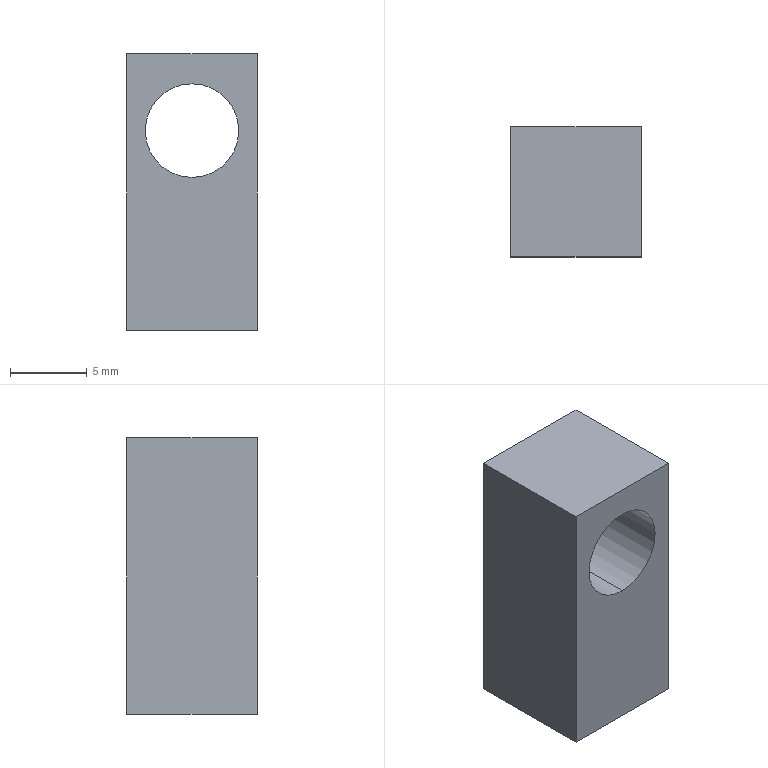Part | STEP file | Buffer mount | 1 solid | 12 faces | box 8.5 x 8.5 x 18 mm | volume 935.428 mm3 | plane 6 | cylinder 4 | cone 2 | commonest cylinder face diameters 4.2 x2 6.1 x2
STEP:
#1=CARTESIAN_POINT('',(0.,0.,0.));
#2=DIRECTION('',(0.,0.,1.));
#3=DIRECTION('',(1.,0.,0.));
#4=AXIS2_PLACEMENT_3D('',#1,#2,#3);
#5=CARTESIAN_POINT('',(2.15,4.25,8.));
#6=VERTEX_POINT('',#5);
#7=CARTESIAN_POINT('',(2.15,4.25,0.));
#8=VERTEX_POINT('',#7);
#9=CARTESIAN_POINT('',(2.15,4.25,0.));
#10=DIRECTION('',(0.,0.,-1.));
#11=VECTOR('',#10,1.);
#12=LINE('',#9,#11);
#13=CARTESIAN_POINT('',(4.25,4.25,0.));
#14=DIRECTION('',(0.,0.,-1.));
#15=DIRECTION('',(-1.,0.,0.));
#16=AXIS2_PLACEMENT_3D('',#13,#14,#15);
#17=CYLINDRICAL_SURFACE('',#16,2.1);
#18=CARTESIAN_POINT('',(6.283,0.));
#19=DIRECTION('',(0.,1.));
#20=VECTOR('',#19,1.);
#21=LINE('',#18,#20);
#22=(GEOMETRIC_REPRESENTATION_CONTEXT(2)PARAMETRIC_REPRESENTATION_CONTEXT()REPRESENTATION_CONTEXT('',''));
#23=DEFINITIONAL_REPRESENTATION('',(#21),#22);
#24=PCURVE('',#17,#23);
#25=CARTESIAN_POINT('',(4.25,4.25,0.));
#26=DIRECTION('',(0.,0.,-1.));
#27=DIRECTION('',(-1.,0.,0.));
#28=AXIS2_PLACEMENT_3D('',#25,#26,#27);
#29=CYLINDRICAL_SURFACE('',#28,2.1);
#30=CARTESIAN_POINT('',(0.,0.));
#31=DIRECTION('',(0.,1.));
#32=VECTOR('',#31,1.);
#33=LINE('',#30,#32);
#34=(GEOMETRIC_REPRESENTATION_CONTEXT(2)PARAMETRIC_REPRESENTATION_CONTEXT()REPRESENTATION_CONTEXT('',''));
#35=DEFINITIONAL_REPRESENTATION('',(#33),#34);
#36=PCURVE('',#29,#35);
#37=SURFACE_CURVE('',#12,(#24,#36),.PCURVE_S1.);
#38=EDGE_CURVE('',#6,#8,#37,.T.);
#39=ORIENTED_EDGE('',*,*,#38,.T.);
#40=CARTESIAN_POINT('',(6.35,4.25,0.));
#41=VERTEX_POINT('',#40);
#42=CARTESIAN_POINT('',(4.25,4.25,0.));
#43=DIRECTION('',(0.,0.,-1.));
#44=DIRECTION('',(-1.,0.,0.));
#45=AXIS2_PLACEMENT_3D('',#42,#43,#44);
#46=CIRCLE('',#45,2.1);
#47=CARTESIAN_POINT('',(0.,0.));
#48=DIRECTION('',(1.,0.));
#49=VECTOR('',#48,1.);
#50=LINE('',#47,#49);
#51=(GEOMETRIC_REPRESENTATION_CONTEXT(2)PARAMETRIC_REPRESENTATION_CONTEXT()REPRESENTATION_CONTEXT('',''));
#52=DEFINITIONAL_REPRESENTATION('',(#50),#51);
#53=PCURVE('',#17,#52);
#54=CARTESIAN_POINT('',(0.,8.5,0.));
#55=DIRECTION('',(0.,0.,-1.));
#56=DIRECTION('',(-1.,0.,0.));
#57=AXIS2_PLACEMENT_3D('',#54,#55,#56);
#58=PLANE('',#57);
#59=CARTESIAN_POINT('',(-4.25,-4.25));
#60=DIRECTION('',(1.,0.));
#61=AXIS2_PLACEMENT_2D('',#59,#60);
#62=CIRCLE('',#61,2.1);
#63=(GEOMETRIC_REPRESENTATION_CONTEXT(2)PARAMETRIC_REPRESENTATION_CONTEXT()REPRESENTATION_CONTEXT('',''));
#64=DEFINITIONAL_REPRESENTATION('',(#62),#63);
#65=PCURVE('',#58,#64);
#66=SURFACE_CURVE('',#46,(#53,#65),.PCURVE_S1.);
#67=EDGE_CURVE('',#41,#8,#66,.T.);
#68=ORIENTED_EDGE('',*,*,#67,.F.);
#69=CARTESIAN_POINT('',(6.35,4.25,8.));
#70=VERTEX_POINT('',#69);
#71=CARTESIAN_POINT('',(6.35,4.25,0.));
#72=DIRECTION('',(0.,0.,-1.));
#73=VECTOR('',#72,1.);
#74=LINE('',#71,#73);
#75=CARTESIAN_POINT('',(3.142,0.));
#76=DIRECTION('',(0.,1.));
#77=VECTOR('',#76,1.);
#78=LINE('',#75,#77);
#79=(GEOMETRIC_REPRESENTATION_CONTEXT(2)PARAMETRIC_REPRESENTATION_CONTEXT()REPRESENTATION_CONTEXT('',''));
#80=DEFINITIONAL_REPRESENTATION('',(#78),#79);
#81=PCURVE('',#17,#80);
#82=CARTESIAN_POINT('',(3.142,0.));
#83=DIRECTION('',(0.,1.));
#84=VECTOR('',#83,1.);
#85=LINE('',#82,#84);
#86=(GEOMETRIC_REPRESENTATION_CONTEXT(2)PARAMETRIC_REPRESENTATION_CONTEXT()REPRESENTATION_CONTEXT('',''));
#87=DEFINITIONAL_REPRESENTATION('',(#85),#86);
#88=PCURVE('',#29,#87);
#89=SURFACE_CURVE('',#74,(#81,#88),.PCURVE_S1.);
#90=EDGE_CURVE('',#70,#41,#89,.T.);
#91=ORIENTED_EDGE('',*,*,#90,.F.);
#92=CARTESIAN_POINT('',(4.25,4.25,8.));
#93=DIRECTION('',(0.,0.,-1.));
#94=DIRECTION('',(-1.,0.,0.));
#95=AXIS2_PLACEMENT_3D('',#92,#93,#94);
#96=CIRCLE('',#95,2.1);
#97=CARTESIAN_POINT('',(0.,-8.));
#98=DIRECTION('',(1.,0.));
#99=VECTOR('',#98,1.);
#100=LINE('',#97,#99);
#101=(GEOMETRIC_REPRESENTATION_CONTEXT(2)PARAMETRIC_REPRESENTATION_CONTEXT()REPRESENTATION_CONTEXT('',''));
#102=DEFINITIONAL_REPRESENTATION('',(#100),#101);
#103=PCURVE('',#17,#102);
#104=CARTESIAN_POINT('',(4.25,4.25,8.));
#105=DIRECTION('',(0.,0.,-1.));
#106=DIRECTION('',(-1.,0.,0.));
#107=AXIS2_PLACEMENT_3D('',#104,#105,#106);
#108=CONICAL_SURFACE('',#107,2.1,1.03);
#109=CARTESIAN_POINT('',(0.,0.));
#110=DIRECTION('',(1.,0.));
#111=VECTOR('',#110,1.);
#112=LINE('',#109,#111);
#113=(GEOMETRIC_REPRESENTATION_CONTEXT(2)PARAMETRIC_REPRESENTATION_CONTEXT()REPRESENTATION_CONTEXT('',''));
#114=DEFINITIONAL_REPRESENTATION('',(#112),#113);
#115=PCURVE('',#108,#114);
#116=SURFACE_CURVE('',#96,(#103,#115),.PCURVE_S1.);
#117=EDGE_CURVE('',#70,#6,#116,.T.);
#118=ORIENTED_EDGE('',*,*,#117,.T.);
#119=EDGE_LOOP('',(#39,#68,#91,#118));
#120=FACE_BOUND('',#119,.F.);
#121=ADVANCED_FACE('',(#120),#17,.F.);
#122=ORIENTED_EDGE('',*,*,#117,.F.);
#123=CARTESIAN_POINT('',(4.25,4.25,9.262));
#124=VERTEX_POINT('',#123);
#125=CARTESIAN_POINT('',(6.35,4.25,8.));
#126=DIRECTION('',(0.8572,0.,-0.515));
#127=VECTOR('',#126,1.);
#128=LINE('',#125,#127);
#129=CARTESIAN_POINT('',(3.142,0.));
#130=DIRECTION('',(0.,1.));
#131=VECTOR('',#130,1.);
#132=LINE('',#129,#131);
#133=(GEOMETRIC_REPRESENTATION_CONTEXT(2)PARAMETRIC_REPRESENTATION_CONTEXT()REPRESENTATION_CONTEXT('',''));
#134=DEFINITIONAL_REPRESENTATION('',(#132),#133);
#135=PCURVE('',#108,#134);
#136=CARTESIAN_POINT('',(4.25,4.25,8.));
#137=DIRECTION('',(0.,0.,-1.));
#138=DIRECTION('',(-1.,0.,0.));
#139=AXIS2_PLACEMENT_3D('',#136,#137,#138);
#140=CONICAL_SURFACE('',#139,2.1,1.03);
#141=CARTESIAN_POINT('',(3.142,0.));
#142=DIRECTION('',(0.,1.));
#143=VECTOR('',#142,1.);
#144=LINE('',#141,#143);
#145=(GEOMETRIC_REPRESENTATION_CONTEXT(2)PARAMETRIC_REPRESENTATION_CONTEXT()REPRESENTATION_CONTEXT('',''));
#146=DEFINITIONAL_REPRESENTATION('',(#144),#145);
#147=PCURVE('',#140,#146);
#148=SURFACE_CURVE('',#128,(#135,#147),.PCURVE_S1.);
#149=EDGE_CURVE('',#124,#70,#148,.T.);
#150=ORIENTED_EDGE('',*,*,#149,.F.);
#151=CARTESIAN_POINT('',(2.15,4.25,8.));
#152=DIRECTION('',(-0.8572,0.,-0.515));
#153=VECTOR('',#152,1.);
#154=LINE('',#151,#153);
#155=CARTESIAN_POINT('',(6.283,0.));
#156=DIRECTION('',(0.,1.));
#157=VECTOR('',#156,1.);
#158=LINE('',#155,#157);
#159=(GEOMETRIC_REPRESENTATION_CONTEXT(2)PARAMETRIC_REPRESENTATION_CONTEXT()REPRESENTATION_CONTEXT('',''));
#160=DEFINITIONAL_REPRESENTATION('',(#158),#159);
#161=PCURVE('',#108,#160);
#162=CARTESIAN_POINT('',(0.,0.));
#163=DIRECTION('',(0.,1.));
#164=VECTOR('',#163,1.);
#165=LINE('',#162,#164);
#166=(GEOMETRIC_REPRESENTATION_CONTEXT(2)PARAMETRIC_REPRESENTATION_CONTEXT()REPRESENTATION_CONTEXT('',''));
#167=DEFINITIONAL_REPRESENTATION('',(#165),#166);
#168=PCURVE('',#140,#167);
#169=SURFACE_CURVE('',#154,(#161,#168),.PCURVE_S1.);
#170=EDGE_CURVE('',#124,#6,#169,.T.);
#171=ORIENTED_EDGE('',*,*,#170,.T.);
#172=EDGE_LOOP('',(#122,#150,#171));
#173=FACE_BOUND('',#172,.F.);
#174=ADVANCED_FACE('',(#173),#108,.F.);
#175=CARTESIAN_POINT('',(4.25,8.5,9.95));
#176=VERTEX_POINT('',#175);
#177=CARTESIAN_POINT('',(4.25,0.,9.95));
#178=VERTEX_POINT('',#177);
#179=CARTESIAN_POINT('',(4.25,8.5,9.95));
#180=DIRECTION('',(0.,-1.,0.));
#181=VECTOR('',#180,1.);
#182=LINE('',#179,#181);
#183=CARTESIAN_POINT('',(4.25,8.5,13.));
#184=DIRECTION('',(0.,-1.,0.));
#185=DIRECTION('',(0.,0.,-1.));
#186=AXIS2_PLACEMENT_3D('',#183,#184,#185);
#187=CYLINDRICAL_SURFACE('',#186,3.05);
#188=CARTESIAN_POINT('',(6.283,0.));
#189=DIRECTION('',(0.,1.));
#190=VECTOR('',#189,1.);
#191=LINE('',#188,#190);
#192=(GEOMETRIC_REPRESENTATION_CONTEXT(2)PARAMETRIC_REPRESENTATION_CONTEXT()REPRESENTATION_CONTEXT('',''));
#193=DEFINITIONAL_REPRESENTATION('',(#191),#192);
#194=PCURVE('',#187,#193);
#195=CARTESIAN_POINT('',(4.25,8.5,13.));
#196=DIRECTION('',(0.,-1.,0.));
#197=DIRECTION('',(0.,0.,-1.));
#198=AXIS2_PLACEMENT_3D('',#195,#196,#197);
#199=CYLINDRICAL_SURFACE('',#198,3.05);
#200=CARTESIAN_POINT('',(0.,0.));
#201=DIRECTION('',(0.,1.));
#202=VECTOR('',#201,1.);
#203=LINE('',#200,#202);
#204=(GEOMETRIC_REPRESENTATION_CONTEXT(2)PARAMETRIC_REPRESENTATION_CONTEXT()REPRESENTATION_CONTEXT('',''));
#205=DEFINITIONAL_REPRESENTATION('',(#203),#204);
#206=PCURVE('',#199,#205);
#207=SURFACE_CURVE('',#182,(#194,#206),.PCURVE_S1.);
#208=EDGE_CURVE('',#176,#178,#207,.T.);
#209=ORIENTED_EDGE('',*,*,#208,.T.);
#210=CARTESIAN_POINT('',(4.25,0.,16.05));
#211=VERTEX_POINT('',#210);
#212=CARTESIAN_POINT('',(4.25,0.,13.));
#213=DIRECTION('',(0.,-1.,0.));
#214=DIRECTION('',(0.,0.,-1.));
#215=AXIS2_PLACEMENT_3D('',#212,#213,#214);
#216=CIRCLE('',#215,3.05);
#217=CARTESIAN_POINT('',(0.,8.5));
#218=DIRECTION('',(1.,0.));
#219=VECTOR('',#218,1.);
#220=LINE('',#217,#219);
#221=(GEOMETRIC_REPRESENTATION_CONTEXT(2)PARAMETRIC_REPRESENTATION_CONTEXT()REPRESENTATION_CONTEXT('',''));
#222=DEFINITIONAL_REPRESENTATION('',(#220),#221);
#223=PCURVE('',#187,#222);
#224=CARTESIAN_POINT('',(0.,0.,18.));
#225=DIRECTION('',(0.,1.,0.));
#226=DIRECTION('',(0.,0.,1.));
#227=AXIS2_PLACEMENT_3D('',#224,#225,#226);
#228=PLANE('',#227);
#229=CARTESIAN_POINT('',(-8.05,4.25));
#230=CARTESIAN_POINT('',(-8.05,9.533));
#231=CARTESIAN_POINT('',(-3.475,6.891));
#232=CARTESIAN_POINT('',(1.1,4.25));
#233=CARTESIAN_POINT('',(-3.475,1.609));
#234=CARTESIAN_POINT('',(-8.05,-1.033));
#235=CARTESIAN_POINT('',(-8.05,4.25));
#236=(BOUNDED_CURVE()B_SPLINE_CURVE(2,(#229,#230,#231,#232,#233,#234,#235),.UNSPECIFIED.,.T.,.F.)B_SPLINE_CURVE_WITH_KNOTS((1,2,2,2,2,1),(-2.094,0.,2.094,4.189,6.283,8.378),.UNSPECIFIED.)CURVE()GEOMETRIC_REPRESENTATION_ITEM()RATIONAL_B_SPLINE_CURVE((1.,0.5,1.,0.5,1.,0.5,1.))REPRESENTATION_ITEM(''));
#237=(GEOMETRIC_REPRESENTATION_CONTEXT(2)PARAMETRIC_REPRESENTATION_CONTEXT()REPRESENTATION_CONTEXT('',''));
#238=DEFINITIONAL_REPRESENTATION('',(#236),#237);
#239=PCURVE('',#228,#238);
#240=SURFACE_CURVE('',#216,(#223,#239),.PCURVE_S1.);
#241=EDGE_CURVE('',#211,#178,#240,.T.);
#242=ORIENTED_EDGE('',*,*,#241,.F.);
#243=CARTESIAN_POINT('',(4.25,8.5,16.05));
#244=VERTEX_POINT('',#243);
#245=CARTESIAN_POINT('',(4.25,8.5,16.05));
#246=DIRECTION('',(0.,-1.,0.));
#247=VECTOR('',#246,1.);
#248=LINE('',#245,#247);
#249=CARTESIAN_POINT('',(3.142,0.));
#250=DIRECTION('',(0.,1.));
#251=VECTOR('',#250,1.);
#252=LINE('',#249,#251);
#253=(GEOMETRIC_REPRESENTATION_CONTEXT(2)PARAMETRIC_REPRESENTATION_CONTEXT()REPRESENTATION_CONTEXT('',''));
#254=DEFINITIONAL_REPRESENTATION('',(#252),#253);
#255=PCURVE('',#187,#254);
#256=CARTESIAN_POINT('',(3.142,0.));
#257=DIRECTION('',(0.,1.));
#258=VECTOR('',#257,1.);
#259=LINE('',#256,#258);
#260=(GEOMETRIC_REPRESENTATION_CONTEXT(2)PARAMETRIC_REPRESENTATION_CONTEXT()REPRESENTATION_CONTEXT('',''));
#261=DEFINITIONAL_REPRESENTATION('',(#259),#260);
#262=PCURVE('',#199,#261);
#263=SURFACE_CURVE('',#248,(#255,#262),.PCURVE_S1.);
#264=EDGE_CURVE('',#244,#211,#263,.T.);
#265=ORIENTED_EDGE('',*,*,#264,.F.);
#266=CARTESIAN_POINT('',(4.25,8.5,13.));
#267=DIRECTION('',(0.,-1.,0.));
#268=DIRECTION('',(0.,0.,-1.));
#269=AXIS2_PLACEMENT_3D('',#266,#267,#268);
#270=CIRCLE('',#269,3.05);
#271=CARTESIAN_POINT('',(0.,0.));
#272=DIRECTION('',(1.,0.));
#273=VECTOR('',#272,1.);
#274=LINE('',#271,#273);
#275=(GEOMETRIC_REPRESENTATION_CONTEXT(2)PARAMETRIC_REPRESENTATION_CONTEXT()REPRESENTATION_CONTEXT('',''));
#276=DEFINITIONAL_REPRESENTATION('',(#274),#275);
#277=PCURVE('',#187,#276);
#278=CARTESIAN_POINT('',(0.,8.5,18.));
#279=DIRECTION('',(0.,-1.,0.));
#280=DIRECTION('',(0.,0.,-1.));
#281=AXIS2_PLACEMENT_3D('',#278,#279,#280);
#282=PLANE('',#281);
#283=CARTESIAN_POINT('',(5.,4.25));
#284=DIRECTION('',(1.,0.));
#285=AXIS2_PLACEMENT_2D('',#283,#284);
#286=CIRCLE('',#285,3.05);
#287=(GEOMETRIC_REPRESENTATION_CONTEXT(2)PARAMETRIC_REPRESENTATION_CONTEXT()REPRESENTATION_CONTEXT('',''));
#288=DEFINITIONAL_REPRESENTATION('',(#286),#287);
#289=PCURVE('',#282,#288);
#290=SURFACE_CURVE('',#270,(#277,#289),.PCURVE_S1.);
#291=EDGE_CURVE('',#244,#176,#290,.T.);
#292=ORIENTED_EDGE('',*,*,#291,.T.);
#293=EDGE_LOOP('',(#209,#242,#265,#292));
#294=FACE_BOUND('',#293,.F.);
#295=ADVANCED_FACE('',(#294),#187,.F.);
#296=CARTESIAN_POINT('',(0.,8.5,0.));
#297=VERTEX_POINT('',#296);
#298=CARTESIAN_POINT('',(0.,0.,0.));
#299=VERTEX_POINT('',#298);
#300=CARTESIAN_POINT('',(0.,0.,0.));
#301=DIRECTION('',(0.,-1.,0.));
#302=VECTOR('',#301,1.);
#303=LINE('',#300,#302);
#304=CARTESIAN_POINT('',(0.,0.,18.));
#305=DIRECTION('',(1.,0.,0.));
#306=DIRECTION('',(0.,1.,0.));
#307=AXIS2_PLACEMENT_3D('',#304,#305,#306);
#308=PLANE('',#307);
#309=CARTESIAN_POINT('',(0.,-18.));
#310=DIRECTION('',(-1.,0.));
#311=VECTOR('',#310,1.);
#312=LINE('',#309,#311);
#313=(GEOMETRIC_REPRESENTATION_CONTEXT(2)PARAMETRIC_REPRESENTATION_CONTEXT()REPRESENTATION_CONTEXT('',''));
#314=DEFINITIONAL_REPRESENTATION('',(#312),#313);
#315=PCURVE('',#308,#314);
#316=CARTESIAN_POINT('',(0.,-8.5));
#317=DIRECTION('',(0.,-1.));
#318=VECTOR('',#317,1.);
#319=LINE('',#316,#318);
#320=(GEOMETRIC_REPRESENTATION_CONTEXT(2)PARAMETRIC_REPRESENTATION_CONTEXT()REPRESENTATION_CONTEXT('',''));
#321=DEFINITIONAL_REPRESENTATION('',(#319),#320);
#322=PCURVE('',#58,#321);
#323=SURFACE_CURVE('',#303,(#315,#322),.PCURVE_S1.);
#324=EDGE_CURVE('',#297,#299,#323,.T.);
#325=ORIENTED_EDGE('',*,*,#324,.T.);
#326=CARTESIAN_POINT('',(0.,0.,18.));
#327=VERTEX_POINT('',#326);
#328=CARTESIAN_POINT('',(0.,0.,18.));
#329=DIRECTION('',(0.,0.,-1.));
#330=VECTOR('',#329,1.);
#331=LINE('',#328,#330);
#332=CARTESIAN_POINT('',(0.,0.));
#333=DIRECTION('',(0.,-1.));
#334=VECTOR('',#333,1.);
#335=LINE('',#332,#334);
#336=(GEOMETRIC_REPRESENTATION_CONTEXT(2)PARAMETRIC_REPRESENTATION_CONTEXT()REPRESENTATION_CONTEXT('',''));
#337=DEFINITIONAL_REPRESENTATION('',(#335),#336);
#338=PCURVE('',#308,#337);
#339=CARTESIAN_POINT('',(0.,0.));
#340=DIRECTION('',(-1.,0.));
#341=VECTOR('',#340,1.);
#342=LINE('',#339,#341);
#343=(GEOMETRIC_REPRESENTATION_CONTEXT(2)PARAMETRIC_REPRESENTATION_CONTEXT()REPRESENTATION_CONTEXT('',''));
#344=DEFINITIONAL_REPRESENTATION('',(#342),#343);
#345=PCURVE('',#228,#344);
#346=SURFACE_CURVE('',#331,(#338,#345),.PCURVE_S1.);
#347=EDGE_CURVE('',#327,#299,#346,.T.);
#348=ORIENTED_EDGE('',*,*,#347,.F.);
#349=CARTESIAN_POINT('',(0.,8.5,18.));
#350=VERTEX_POINT('',#349);
#351=CARTESIAN_POINT('',(0.,0.,18.));
#352=DIRECTION('',(0.,-1.,0.));
#353=VECTOR('',#352,1.);
#354=LINE('',#351,#353);
#355=CARTESIAN_POINT('',(0.,0.));
#356=DIRECTION('',(-1.,0.));
#357=VECTOR('',#356,1.);
#358=LINE('',#355,#357);
#359=(GEOMETRIC_REPRESENTATION_CONTEXT(2)PARAMETRIC_REPRESENTATION_CONTEXT()REPRESENTATION_CONTEXT('',''));
#360=DEFINITIONAL_REPRESENTATION('',(#358),#359);
#361=PCURVE('',#308,#360);
#362=CARTESIAN_POINT('',(0.,8.5,18.));
#363=DIRECTION('',(0.,0.,-1.));
#364=DIRECTION('',(-1.,0.,0.));
#365=AXIS2_PLACEMENT_3D('',#362,#363,#364);
#366=PLANE('',#365);
#367=CARTESIAN_POINT('',(0.,-8.5));
#368=DIRECTION('',(0.,-1.));
#369=VECTOR('',#368,1.);
#370=LINE('',#367,#369);
#371=(GEOMETRIC_REPRESENTATION_CONTEXT(2)PARAMETRIC_REPRESENTATION_CONTEXT()REPRESENTATION_CONTEXT('',''));
#372=DEFINITIONAL_REPRESENTATION('',(#370),#371);
#373=PCURVE('',#366,#372);
#374=SURFACE_CURVE('',#354,(#361,#373),.PCURVE_S1.);
#375=EDGE_CURVE('',#350,#327,#374,.T.);
#376=ORIENTED_EDGE('',*,*,#375,.F.);
#377=CARTESIAN_POINT('',(0.,8.5,18.));
#378=DIRECTION('',(0.,0.,-1.));
#379=VECTOR('',#378,1.);
#380=LINE('',#377,#379);
#381=CARTESIAN_POINT('',(8.5,0.));
#382=DIRECTION('',(0.,-1.));
#383=VECTOR('',#382,1.);
#384=LINE('',#381,#383);
#385=(GEOMETRIC_REPRESENTATION_CONTEXT(2)PARAMETRIC_REPRESENTATION_CONTEXT()REPRESENTATION_CONTEXT('',''));
#386=DEFINITIONAL_REPRESENTATION('',(#384),#385);
#387=PCURVE('',#308,#386);
#388=CARTESIAN_POINT('',(0.,0.));
#389=DIRECTION('',(1.,0.));
#390=VECTOR('',#389,1.);
#391=LINE('',#388,#390);
#392=(GEOMETRIC_REPRESENTATION_CONTEXT(2)PARAMETRIC_REPRESENTATION_CONTEXT()REPRESENTATION_CONTEXT('',''));
#393=DEFINITIONAL_REPRESENTATION('',(#391),#392);
#394=PCURVE('',#282,#393);
#395=SURFACE_CURVE('',#380,(#387,#394),.PCURVE_S1.);
#396=EDGE_CURVE('',#350,#297,#395,.T.);
#397=ORIENTED_EDGE('',*,*,#396,.T.);
#398=EDGE_LOOP('',(#325,#348,#376,#397));
#399=FACE_BOUND('',#398,.T.);
#400=ADVANCED_FACE('',(#399),#308,.F.);
#401=CARTESIAN_POINT('',(4.25,0.,13.));
#402=DIRECTION('',(0.,-1.,0.));
#403=DIRECTION('',(0.,0.,-1.));
#404=AXIS2_PLACEMENT_3D('',#401,#402,#403);
#405=CIRCLE('',#404,3.05);
#406=CARTESIAN_POINT('',(-8.05,4.25));
#407=CARTESIAN_POINT('',(-8.05,9.533));
#408=CARTESIAN_POINT('',(-3.475,6.891));
#409=CARTESIAN_POINT('',(1.1,4.25));
#410=CARTESIAN_POINT('',(-3.475,1.609));
#411=CARTESIAN_POINT('',(-8.05,-1.033));
#412=CARTESIAN_POINT('',(-8.05,4.25));
#413=(BOUNDED_CURVE()B_SPLINE_CURVE(2,(#406,#407,#408,#409,#410,#411,#412),.UNSPECIFIED.,.T.,.F.)B_SPLINE_CURVE_WITH_KNOTS((1,2,2,2,2,1),(-2.094,0.,2.094,4.189,6.283,8.378),.UNSPECIFIED.)CURVE()GEOMETRIC_REPRESENTATION_ITEM()RATIONAL_B_SPLINE_CURVE((1.,0.5,1.,0.5,1.,0.5,1.))REPRESENTATION_ITEM(''));
#414=(GEOMETRIC_REPRESENTATION_CONTEXT(2)PARAMETRIC_REPRESENTATION_CONTEXT()REPRESENTATION_CONTEXT('',''));
#415=DEFINITIONAL_REPRESENTATION('',(#413),#414);
#416=PCURVE('',#228,#415);
#417=CARTESIAN_POINT('',(0.,8.5));
#418=DIRECTION('',(1.,0.));
#419=VECTOR('',#418,1.);
#420=LINE('',#417,#419);
#421=(GEOMETRIC_REPRESENTATION_CONTEXT(2)PARAMETRIC_REPRESENTATION_CONTEXT()REPRESENTATION_CONTEXT('',''));
#422=DEFINITIONAL_REPRESENTATION('',(#420),#421);
#423=PCURVE('',#199,#422);
#424=SURFACE_CURVE('',#405,(#416,#423),.PCURVE_S1.);
#425=EDGE_CURVE('',#178,#211,#424,.T.);
#426=ORIENTED_EDGE('',*,*,#425,.F.);
#427=ORIENTED_EDGE('',*,*,#241,.F.);
#428=EDGE_LOOP('',(#426,#427));
#429=FACE_BOUND('',#428,.T.);
#430=CARTESIAN_POINT('',(8.5,0.,0.));
#431=VERTEX_POINT('',#430);
#432=CARTESIAN_POINT('',(0.,0.,0.));
#433=DIRECTION('',(1.,0.,0.));
#434=VECTOR('',#433,1.);
#435=LINE('',#432,#434);
#436=CARTESIAN_POINT('',(-18.,0.));
#437=DIRECTION('',(0.,1.));
#438=VECTOR('',#437,1.);
#439=LINE('',#436,#438);
#440=(GEOMETRIC_REPRESENTATION_CONTEXT(2)PARAMETRIC_REPRESENTATION_CONTEXT()REPRESENTATION_CONTEXT('',''));
#441=DEFINITIONAL_REPRESENTATION('',(#439),#440);
#442=PCURVE('',#228,#441);
#443=CARTESIAN_POINT('',(0.,-8.5));
#444=DIRECTION('',(-1.,0.));
#445=VECTOR('',#444,1.);
#446=LINE('',#443,#445);
#447=(GEOMETRIC_REPRESENTATION_CONTEXT(2)PARAMETRIC_REPRESENTATION_CONTEXT()REPRESENTATION_CONTEXT('',''));
#448=DEFINITIONAL_REPRESENTATION('',(#446),#447);
#449=PCURVE('',#58,#448);
#450=SURFACE_CURVE('',#435,(#442,#449),.PCURVE_S1.);
#451=EDGE_CURVE('',#299,#431,#450,.T.);
#452=ORIENTED_EDGE('',*,*,#451,.T.);
#453=CARTESIAN_POINT('',(8.5,0.,18.));
#454=VERTEX_POINT('',#453);
#455=CARTESIAN_POINT('',(8.5,0.,18.));
#456=DIRECTION('',(0.,0.,-1.));
#457=VECTOR('',#456,1.);
#458=LINE('',#455,#457);
#459=CARTESIAN_POINT('',(0.,8.5));
#460=DIRECTION('',(-1.,0.));
#461=VECTOR('',#460,1.);
#462=LINE('',#459,#461);
#463=(GEOMETRIC_REPRESENTATION_CONTEXT(2)PARAMETRIC_REPRESENTATION_CONTEXT()REPRESENTATION_CONTEXT('',''));
#464=DEFINITIONAL_REPRESENTATION('',(#462),#463);
#465=PCURVE('',#228,#464);
#466=CARTESIAN_POINT('',(8.5,0.,18.));
#467=DIRECTION('',(-1.,0.,0.));
#468=DIRECTION('',(0.,-1.,0.));
#469=AXIS2_PLACEMENT_3D('',#466,#467,#468);
#470=PLANE('',#469);
#471=CARTESIAN_POINT('',(0.,0.));
#472=DIRECTION('',(0.,-1.));
#473=VECTOR('',#472,1.);
#474=LINE('',#471,#473);
#475=(GEOMETRIC_REPRESENTATION_CONTEXT(2)PARAMETRIC_REPRESENTATION_CONTEXT()REPRESENTATION_CONTEXT('',''));
#476=DEFINITIONAL_REPRESENTATION('',(#474),#475);
#477=PCURVE('',#470,#476);
#478=SURFACE_CURVE('',#458,(#465,#477),.PCURVE_S1.);
#479=EDGE_CURVE('',#454,#431,#478,.T.);
#480=ORIENTED_EDGE('',*,*,#479,.F.);
#481=CARTESIAN_POINT('',(0.,0.,18.));
#482=DIRECTION('',(1.,0.,0.));
#483=VECTOR('',#482,1.);
#484=LINE('',#481,#483);
#485=CARTESIAN_POINT('',(0.,0.));
#486=DIRECTION('',(0.,1.));
#487=VECTOR('',#486,1.);
#488=LINE('',#485,#487);
#489=(GEOMETRIC_REPRESENTATION_CONTEXT(2)PARAMETRIC_REPRESENTATION_CONTEXT()REPRESENTATION_CONTEXT('',''));
#490=DEFINITIONAL_REPRESENTATION('',(#488),#489);
#491=PCURVE('',#228,#490);
#492=CARTESIAN_POINT('',(0.,-8.5));
#493=DIRECTION('',(-1.,0.));
#494=VECTOR('',#493,1.);
#495=LINE('',#492,#494);
#496=(GEOMETRIC_REPRESENTATION_CONTEXT(2)PARAMETRIC_REPRESENTATION_CONTEXT()REPRESENTATION_CONTEXT('',''));
#497=DEFINITIONAL_REPRESENTATION('',(#495),#496);
#498=PCURVE('',#366,#497);
#499=SURFACE_CURVE('',#484,(#491,#498),.PCURVE_S1.);
#500=EDGE_CURVE('',#327,#454,#499,.T.);
#501=ORIENTED_EDGE('',*,*,#500,.F.);
#502=ORIENTED_EDGE('',*,*,#347,.T.);
#503=EDGE_LOOP('',(#452,#480,#501,#502));
#504=FACE_BOUND('',#503,.T.);
#505=ADVANCED_FACE('',(#429,#504),#228,.F.);
#506=CARTESIAN_POINT('',(8.5,8.5,0.));
#507=VERTEX_POINT('',#506);
#508=CARTESIAN_POINT('',(8.5,0.,0.));
#509=DIRECTION('',(0.,1.,0.));
#510=VECTOR('',#509,1.);
#511=LINE('',#508,#510);
#512=CARTESIAN_POINT('',(0.,-18.));
#513=DIRECTION('',(-1.,0.));
#514=VECTOR('',#513,1.);
#515=LINE('',#512,#514);
#516=(GEOMETRIC_REPRESENTATION_CONTEXT(2)PARAMETRIC_REPRESENTATION_CONTEXT()REPRESENTATION_CONTEXT('',''));
#517=DEFINITIONAL_REPRESENTATION('',(#515),#516);
#518=PCURVE('',#470,#517);
#519=CARTESIAN_POINT('',(-8.5,-8.5));
#520=DIRECTION('',(0.,1.));
#521=VECTOR('',#520,1.);
#522=LINE('',#519,#521);
#523=(GEOMETRIC_REPRESENTATION_CONTEXT(2)PARAMETRIC_REPRESENTATION_CONTEXT()REPRESENTATION_CONTEXT('',''));
#524=DEFINITIONAL_REPRESENTATION('',(#522),#523);
#525=PCURVE('',#58,#524);
#526=SURFACE_CURVE('',#511,(#518,#525),.PCURVE_S1.);
#527=EDGE_CURVE('',#431,#507,#526,.T.);
#528=ORIENTED_EDGE('',*,*,#527,.T.);
#529=CARTESIAN_POINT('',(8.5,8.5,18.));
#530=VERTEX_POINT('',#529);
#531=CARTESIAN_POINT('',(8.5,8.5,18.));
#532=DIRECTION('',(0.,0.,-1.));
#533=VECTOR('',#532,1.);
#534=LINE('',#531,#533);
#535=CARTESIAN_POINT('',(-8.5,0.));
#536=DIRECTION('',(0.,-1.));
#537=VECTOR('',#536,1.);
#538=LINE('',#535,#537);
#539=(GEOMETRIC_REPRESENTATION_CONTEXT(2)PARAMETRIC_REPRESENTATION_CONTEXT()REPRESENTATION_CONTEXT('',''));
#540=DEFINITIONAL_REPRESENTATION('',(#538),#539);
#541=PCURVE('',#470,#540);
#542=CARTESIAN_POINT('',(0.,8.5));
#543=DIRECTION('',(1.,0.));
#544=VECTOR('',#543,1.);
#545=LINE('',#542,#544);
#546=(GEOMETRIC_REPRESENTATION_CONTEXT(2)PARAMETRIC_REPRESENTATION_CONTEXT()REPRESENTATION_CONTEXT('',''));
#547=DEFINITIONAL_REPRESENTATION('',(#545),#546);
#548=PCURVE('',#282,#547);
#549=SURFACE_CURVE('',#534,(#541,#548),.PCURVE_S1.);
#550=EDGE_CURVE('',#530,#507,#549,.T.);
#551=ORIENTED_EDGE('',*,*,#550,.F.);
#552=CARTESIAN_POINT('',(8.5,0.,18.));
#553=DIRECTION('',(0.,1.,0.));
#554=VECTOR('',#553,1.);
#555=LINE('',#552,#554);
#556=CARTESIAN_POINT('',(0.,0.));
#557=DIRECTION('',(-1.,0.));
#558=VECTOR('',#557,1.);
#559=LINE('',#556,#558);
#560=(GEOMETRIC_REPRESENTATION_CONTEXT(2)PARAMETRIC_REPRESENTATION_CONTEXT()REPRESENTATION_CONTEXT('',''));
#561=DEFINITIONAL_REPRESENTATION('',(#559),#560);
#562=PCURVE('',#470,#561);
#563=CARTESIAN_POINT('',(-8.5,-8.5));
#564=DIRECTION('',(0.,1.));
#565=VECTOR('',#564,1.);
#566=LINE('',#563,#565);
#567=(GEOMETRIC_REPRESENTATION_CONTEXT(2)PARAMETRIC_REPRESENTATION_CONTEXT()REPRESENTATION_CONTEXT('',''));
#568=DEFINITIONAL_REPRESENTATION('',(#566),#567);
#569=PCURVE('',#366,#568);
#570=SURFACE_CURVE('',#555,(#562,#569),.PCURVE_S1.);
#571=EDGE_CURVE('',#454,#530,#570,.T.);
#572=ORIENTED_EDGE('',*,*,#571,.F.);
#573=ORIENTED_EDGE('',*,*,#479,.T.);
#574=EDGE_LOOP('',(#528,#551,#572,#573));
#575=FACE_BOUND('',#574,.T.);
#576=ADVANCED_FACE('',(#575),#470,.F.);
#577=CARTESIAN_POINT('',(4.25,8.5,13.));
#578=DIRECTION('',(0.,-1.,0.));
#579=DIRECTION('',(0.,0.,-1.));
#580=AXIS2_PLACEMENT_3D('',#577,#578,#579);
#581=CIRCLE('',#580,3.05);
#582=CARTESIAN_POINT('',(5.,4.25));
#583=DIRECTION('',(1.,0.));
#584=AXIS2_PLACEMENT_2D('',#582,#583);
#585=CIRCLE('',#584,3.05);
#586=(GEOMETRIC_REPRESENTATION_CONTEXT(2)PARAMETRIC_REPRESENTATION_CONTEXT()REPRESENTATION_CONTEXT('',''));
#587=DEFINITIONAL_REPRESENTATION('',(#585),#586);
#588=PCURVE('',#282,#587);
#589=CARTESIAN_POINT('',(0.,0.));
#590=DIRECTION('',(1.,0.));
#591=VECTOR('',#590,1.);
#592=LINE('',#589,#591);
#593=(GEOMETRIC_REPRESENTATION_CONTEXT(2)PARAMETRIC_REPRESENTATION_CONTEXT()REPRESENTATION_CONTEXT('',''));
#594=DEFINITIONAL_REPRESENTATION('',(#592),#593);
#595=PCURVE('',#199,#594);
#596=SURFACE_CURVE('',#581,(#588,#595),.PCURVE_S1.);
#597=EDGE_CURVE('',#176,#244,#596,.T.);
#598=ORIENTED_EDGE('',*,*,#597,.T.);
#599=ORIENTED_EDGE('',*,*,#291,.T.);
#600=EDGE_LOOP('',(#598,#599));
#601=FACE_BOUND('',#600,.T.);
#602=CARTESIAN_POINT('',(0.,8.5,0.));
#603=DIRECTION('',(-1.,0.,0.));
#604=VECTOR('',#603,1.);
#605=LINE('',#602,#604);
#606=CARTESIAN_POINT('',(18.,0.));
#607=DIRECTION('',(0.,-1.));
#608=VECTOR('',#607,1.);
#609=LINE('',#606,#608);
#610=(GEOMETRIC_REPRESENTATION_CONTEXT(2)PARAMETRIC_REPRESENTATION_CONTEXT()REPRESENTATION_CONTEXT('',''));
#611=DEFINITIONAL_REPRESENTATION('',(#609),#610);
#612=PCURVE('',#282,#611);
#613=CARTESIAN_POINT('',(0.,0.));
#614=DIRECTION('',(1.,0.));
#615=VECTOR('',#614,1.);
#616=LINE('',#613,#615);
#617=(GEOMETRIC_REPRESENTATION_CONTEXT(2)PARAMETRIC_REPRESENTATION_CONTEXT()REPRESENTATION_CONTEXT('',''));
#618=DEFINITIONAL_REPRESENTATION('',(#616),#617);
#619=PCURVE('',#58,#618);
#620=SURFACE_CURVE('',#605,(#612,#619),.PCURVE_S1.);
#621=EDGE_CURVE('',#507,#297,#620,.T.);
#622=ORIENTED_EDGE('',*,*,#621,.T.);
#623=ORIENTED_EDGE('',*,*,#396,.F.);
#624=CARTESIAN_POINT('',(0.,8.5,18.));
#625=DIRECTION('',(-1.,0.,0.));
#626=VECTOR('',#625,1.);
#627=LINE('',#624,#626);
#628=CARTESIAN_POINT('',(0.,0.));
#629=DIRECTION('',(0.,-1.));
#630=VECTOR('',#629,1.);
#631=LINE('',#628,#630);
#632=(GEOMETRIC_REPRESENTATION_CONTEXT(2)PARAMETRIC_REPRESENTATION_CONTEXT()REPRESENTATION_CONTEXT('',''));
#633=DEFINITIONAL_REPRESENTATION('',(#631),#632);
#634=PCURVE('',#282,#633);
#635=CARTESIAN_POINT('',(0.,0.));
#636=DIRECTION('',(1.,0.));
#637=VECTOR('',#636,1.);
#638=LINE('',#635,#637);
#639=(GEOMETRIC_REPRESENTATION_CONTEXT(2)PARAMETRIC_REPRESENTATION_CONTEXT()REPRESENTATION_CONTEXT('',''));
#640=DEFINITIONAL_REPRESENTATION('',(#638),#639);
#641=PCURVE('',#366,#640);
#642=SURFACE_CURVE('',#627,(#634,#641),.PCURVE_S1.);
#643=EDGE_CURVE('',#530,#350,#642,.T.);
#644=ORIENTED_EDGE('',*,*,#643,.F.);
#645=ORIENTED_EDGE('',*,*,#550,.T.);
#646=EDGE_LOOP('',(#622,#623,#644,#645));
#647=FACE_BOUND('',#646,.T.);
#648=ADVANCED_FACE('',(#601,#647),#282,.F.);
#649=ORIENTED_EDGE('',*,*,#375,.T.);
#650=ORIENTED_EDGE('',*,*,#500,.T.);
#651=ORIENTED_EDGE('',*,*,#571,.T.);
#652=ORIENTED_EDGE('',*,*,#643,.T.);
#653=EDGE_LOOP('',(#649,#650,#651,#652));
#654=FACE_BOUND('',#653,.T.);
#655=ADVANCED_FACE('',(#654),#366,.F.);
#656=CARTESIAN_POINT('',(4.25,4.25,0.));
#657=DIRECTION('',(0.,0.,-1.));
#658=DIRECTION('',(-1.,0.,0.));
#659=AXIS2_PLACEMENT_3D('',#656,#657,#658);
#660=CIRCLE('',#659,2.1);
#661=CARTESIAN_POINT('',(-4.25,-4.25));
#662=DIRECTION('',(1.,0.));
#663=AXIS2_PLACEMENT_2D('',#661,#662);
#664=CIRCLE('',#663,2.1);
#665=(GEOMETRIC_REPRESENTATION_CONTEXT(2)PARAMETRIC_REPRESENTATION_CONTEXT()REPRESENTATION_CONTEXT('',''));
#666=DEFINITIONAL_REPRESENTATION('',(#664),#665);
#667=PCURVE('',#58,#666);
#668=CARTESIAN_POINT('',(0.,0.));
#669=DIRECTION('',(1.,0.));
#670=VECTOR('',#669,1.);
#671=LINE('',#668,#670);
#672=(GEOMETRIC_REPRESENTATION_CONTEXT(2)PARAMETRIC_REPRESENTATION_CONTEXT()REPRESENTATION_CONTEXT('',''));
#673=DEFINITIONAL_REPRESENTATION('',(#671),#672);
#674=PCURVE('',#29,#673);
#675=SURFACE_CURVE('',#660,(#667,#674),.PCURVE_S1.);
#676=EDGE_CURVE('',#8,#41,#675,.T.);
#677=ORIENTED_EDGE('',*,*,#676,.F.);
#678=ORIENTED_EDGE('',*,*,#67,.F.);
#679=EDGE_LOOP('',(#677,#678));
#680=FACE_BOUND('',#679,.T.);
#681=ORIENTED_EDGE('',*,*,#324,.F.);
#682=ORIENTED_EDGE('',*,*,#621,.F.);
#683=ORIENTED_EDGE('',*,*,#527,.F.);
#684=ORIENTED_EDGE('',*,*,#451,.F.);
#685=EDGE_LOOP('',(#681,#682,#683,#684));
#686=FACE_BOUND('',#685,.T.);
#687=ADVANCED_FACE('',(#680,#686),#58,.T.);
#688=ORIENTED_EDGE('',*,*,#425,.F.);
#689=ORIENTED_EDGE('',*,*,#208,.F.);
#690=ORIENTED_EDGE('',*,*,#597,.T.);
#691=ORIENTED_EDGE('',*,*,#264,.T.);
#692=EDGE_LOOP('',(#688,#689,#690,#691));
#693=FACE_BOUND('',#692,.F.);
#694=ADVANCED_FACE('',(#693),#199,.F.);
#695=CARTESIAN_POINT('',(4.25,4.25,8.));
#696=DIRECTION('',(0.,0.,-1.));
#697=DIRECTION('',(-1.,0.,0.));
#698=AXIS2_PLACEMENT_3D('',#695,#696,#697);
#699=CIRCLE('',#698,2.1);
#700=CARTESIAN_POINT('',(0.,0.));
#701=DIRECTION('',(1.,0.));
#702=VECTOR('',#701,1.);
#703=LINE('',#700,#702);
#704=(GEOMETRIC_REPRESENTATION_CONTEXT(2)PARAMETRIC_REPRESENTATION_CONTEXT()REPRESENTATION_CONTEXT('',''));
#705=DEFINITIONAL_REPRESENTATION('',(#703),#704);
#706=PCURVE('',#140,#705);
#707=CARTESIAN_POINT('',(0.,-8.));
#708=DIRECTION('',(1.,0.));
#709=VECTOR('',#708,1.);
#710=LINE('',#707,#709);
#711=(GEOMETRIC_REPRESENTATION_CONTEXT(2)PARAMETRIC_REPRESENTATION_CONTEXT()REPRESENTATION_CONTEXT('',''));
#712=DEFINITIONAL_REPRESENTATION('',(#710),#711);
#713=PCURVE('',#29,#712);
#714=SURFACE_CURVE('',#699,(#706,#713),.PCURVE_S1.);
#715=EDGE_CURVE('',#6,#70,#714,.T.);
#716=ORIENTED_EDGE('',*,*,#715,.F.);
#717=ORIENTED_EDGE('',*,*,#170,.F.);
#718=ORIENTED_EDGE('',*,*,#149,.T.);
#719=EDGE_LOOP('',(#716,#717,#718));
#720=FACE_BOUND('',#719,.F.);
#721=ADVANCED_FACE('',(#720),#140,.F.);
#722=ORIENTED_EDGE('',*,*,#676,.F.);
#723=ORIENTED_EDGE('',*,*,#38,.F.);
#724=ORIENTED_EDGE('',*,*,#715,.T.);
#725=ORIENTED_EDGE('',*,*,#90,.T.);
#726=EDGE_LOOP('',(#722,#723,#724,#725));
#727=FACE_BOUND('',#726,.F.);
#728=ADVANCED_FACE('',(#727),#29,.F.);
#729=CLOSED_SHELL('',(#121,#174,#295,#400,#505,#576,#648,#655,#687,#694,#721,#728));
#730=MANIFOLD_SOLID_BREP('',#729);
#731=(LENGTH_UNIT()NAMED_UNIT(*)SI_UNIT(.MILLI.,.METRE.));
#732=UNCERTAINTY_MEASURE_WITH_UNIT(LENGTH_MEASURE(0.0000001),#731,'','');
#733=(NAMED_UNIT(*)PLANE_ANGLE_UNIT()SI_UNIT($,.RADIAN.));
#734=(NAMED_UNIT(*)SI_UNIT($,.STERADIAN.)SOLID_ANGLE_UNIT());
#735=(GEOMETRIC_REPRESENTATION_CONTEXT(3)GLOBAL_UNCERTAINTY_ASSIGNED_CONTEXT((#732))GLOBAL_UNIT_ASSIGNED_CONTEXT((#731,#733,#734))REPRESENTATION_CONTEXT('',''));
#736=ADVANCED_BREP_SHAPE_REPRESENTATION('',(#4,#730),#735);